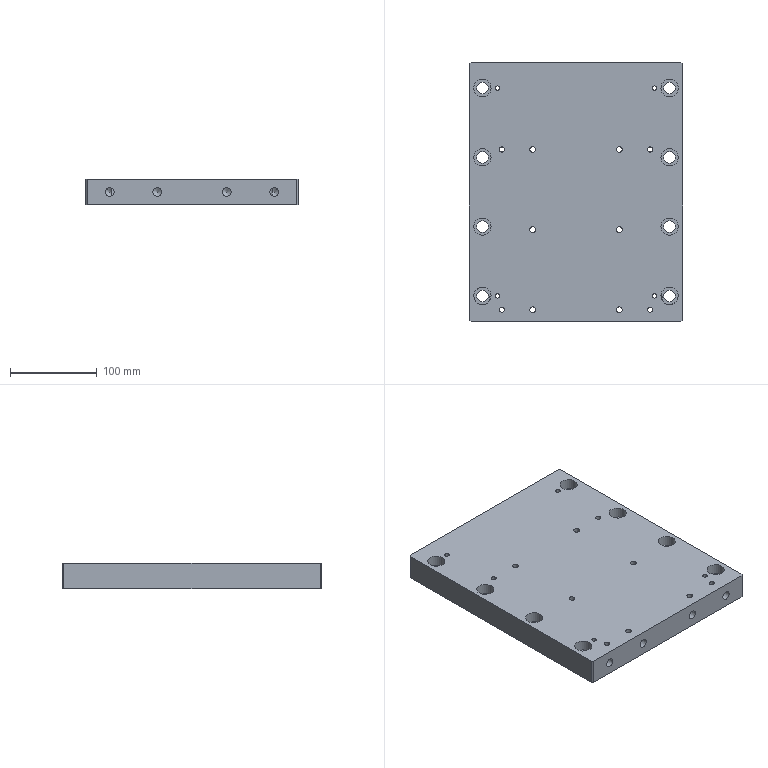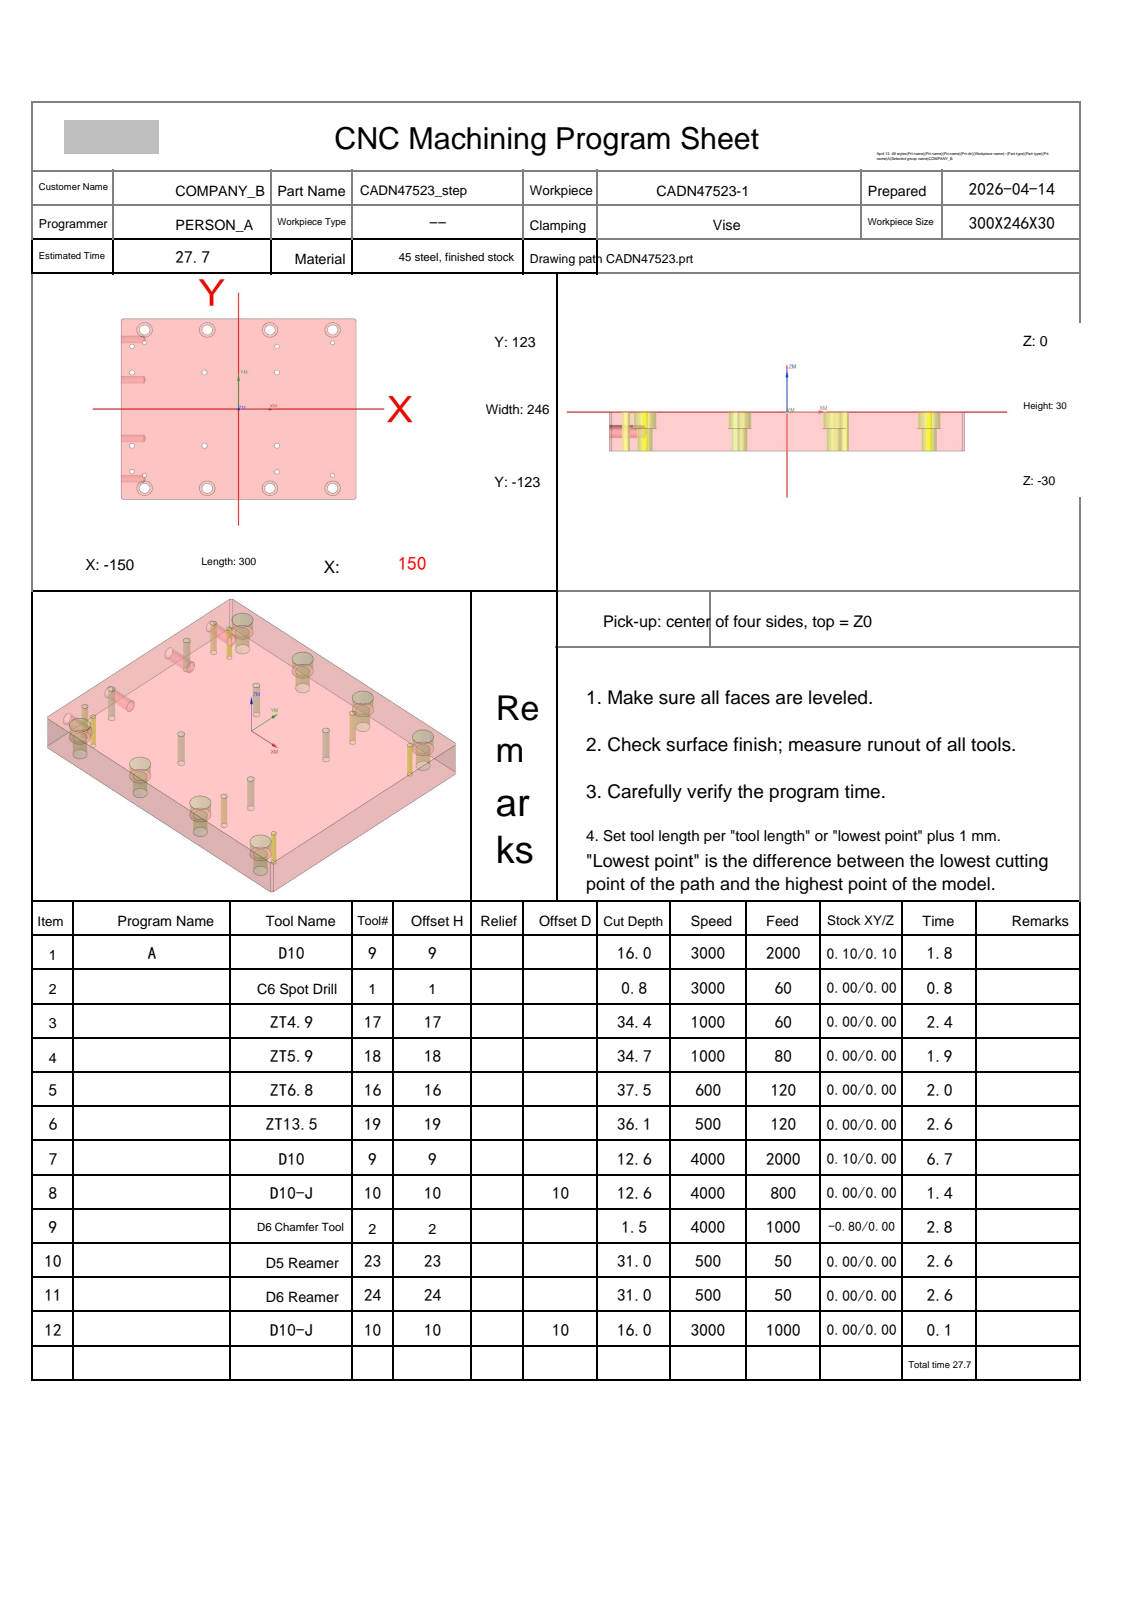NC program | NX | posted by the shop | part box 246 x 300 x 30 mm
Whole program, first 1647 of 1998 lines:
%
O0001
(Machine time: 29.90 MIN)
(===Total Tool:10===)
(T9=D10     D=10.  R=0.   D-  H09 Z=-16.  )
(T1=C6 Spot Drill   D=6.   R=0.   D-  H01 Z=-0.8  )
(T17=ZT4.9  D=4.9  DR_a=120 D-  H17 Z=-34.41)
(T18=ZT5.9  D=5.9  DR_a=120 D-  H18 Z=-34.7 )
(T16=ZT6.8  D=6.8  DR_a=118 D-  H16 Z=-37.54)
(T19=ZT13.5 D=13.5 DR_a=118 D-  H19 Z=-36.06)
(T10=D10-J  D=10.  R=0.   D10 H10 Z=-16.  )
(T2=D6 Chamfer Tool   D=6.   R=0.   D-  H02 Z=-1.5  )
(T23=D5 Reamer   D=5.   DR_a=180 D-  H23 Z=-31.  )
(T24=D6 Reamer   D=6.   DR_a=180 D-  H24 Z=-31.  )
G80 G90 G17 G49 G40
G91 G28 Z0
M01
N1 T09 M06
(D10  D=10. R=0. H=09 ce=0.10 di=0.10)
G00 G90 G54 X145.112 Y133.1 M03 S3000
G43 H09 Z20.
M08
Z-.4
G01 X151.606 Y126.606 F2000.
X153.606 Y124.606
X160.1 Y118.112
G00 Z-.8
G01 X153.606 Y124.606
X151.606 Y126.606
X145.112 Y133.1
G00 Z-1.2
G01 X151.606 Y126.606
X153.606 Y124.606
X160.1 Y118.112
G00 Z-1.6
G01 X153.606 Y124.606
X151.606 Y126.606
X145.112 Y133.1
G00 Z-2.
G01 X151.606 Y126.606
X153.606 Y124.606
X160.1 Y118.112
G00 Z-2.4
G01 X153.606 Y124.606
X151.606 Y126.606
X145.112 Y133.1
G00 Z-2.8
G01 X151.606 Y126.606
X153.606 Y124.606
X160.1 Y118.112
G00 Z-3.2
G01 X153.606 Y124.606
X151.606 Y126.606
X145.112 Y133.1
G00 Z-3.6
G01 X151.606 Y126.606
X153.606 Y124.606
X160.1 Y118.112
G00 Z-4.
G01 X153.606 Y124.606
X151.606 Y126.606
X145.112 Y133.1
G00 Z-4.4
G01 X151.606 Y126.606
X153.606 Y124.606
X160.1 Y118.112
G00 Z-4.8
G01 X153.606 Y124.606
X151.606 Y126.606
X145.112 Y133.1
G00 Z-5.2
G01 X151.606 Y126.606
X153.606 Y124.606
X160.1 Y118.112
G00 Z-5.6
G01 X153.606 Y124.606
X151.606 Y126.606
X145.112 Y133.1
G00 Z-6.
G01 X151.606 Y126.606
X153.606 Y124.606
X160.1 Y118.112
G00 Z-6.4
G01 X153.606 Y124.606
X151.606 Y126.606
X145.112 Y133.1
G00 Z-6.8
G01 X151.606 Y126.606
X153.606 Y124.606
X160.1 Y118.112
G00 Z-7.2
G01 X153.606 Y124.606
X151.606 Y126.606
X145.112 Y133.1
G00 Z-7.6
G01 X151.606 Y126.606
X153.606 Y124.606
X160.1 Y118.112
G00 Z-8.
G01 X153.606 Y124.606
X151.606 Y126.606
X145.112 Y133.1
G00 Z-8.4
G01 X151.606 Y126.606
X153.606 Y124.606
X160.1 Y118.112
G00 Z-8.8
G01 X153.606 Y124.606
X151.606 Y126.606
X145.112 Y133.1
G00 Z-9.2
G01 X151.606 Y126.606
X153.606 Y124.606
X160.1 Y118.112
G00 Z-9.6
G01 X153.606 Y124.606
X151.606 Y126.606
X145.112 Y133.1
G00 Z-10.
G01 X151.606 Y126.606
X153.606 Y124.606
X160.1 Y118.112
G00 Z-10.4
G01 X153.606 Y124.606
X151.606 Y126.606
X145.112 Y133.1
G00 Z-10.8
G01 X151.606 Y126.606
X153.606 Y124.606
X160.1 Y118.112
G00 Z-11.2
G01 X153.606 Y124.606
X151.606 Y126.606
X145.112 Y133.1
G00 Z-11.6
G01 X151.606 Y126.606
X153.606 Y124.606
X160.1 Y118.112
G00 Z-12.
G01 X153.606 Y124.606
X151.606 Y126.606
X145.112 Y133.1
G00 Z-12.4
G01 X151.606 Y126.606
X153.606 Y124.606
X160.1 Y118.112
G00 Z-12.8
G01 X153.606 Y124.606
X151.606 Y126.606
X145.112 Y133.1
G00 Z-13.2
G01 X151.606 Y126.606
X153.606 Y124.606
X160.1 Y118.112
G00 Z-13.6
G01 X153.606 Y124.606
X151.606 Y126.606
X145.112 Y133.1
G00 Z-14.
G01 X151.606 Y126.606
X153.606 Y124.606
X160.1 Y118.112
G00 Z-14.4
G01 X153.606 Y124.606
X151.606 Y126.606
X145.112 Y133.1
G00 Z-14.8
G01 X151.606 Y126.606
X153.606 Y124.606
X160.1 Y118.112
G00 Z-15.2
G01 X153.606 Y124.606
X151.606 Y126.606
X145.112 Y133.1
G00 Z-15.6
G01 X151.606 Y126.606
X153.606 Y124.606
X160.1 Y118.112
G00 Z-16.
G01 X153.606 Y124.606
X151.606 Y126.606
X145.112 Y133.1
G00 Z20.
X160.1 Y-118.112
Z-.4
G01 X153.606 Y-124.606
X151.606 Y-126.606
X145.112 Y-133.1
G00 Z-.8
G01 X151.606 Y-126.606
X153.606 Y-124.606
X160.1 Y-118.112
G00 Z-1.2
G01 X153.606 Y-124.606
X151.606 Y-126.606
X145.112 Y-133.1
G00 Z-1.6
G01 X151.606 Y-126.606
X153.606 Y-124.606
X160.1 Y-118.112
G00 Z-2.
G01 X153.606 Y-124.606
X151.606 Y-126.606
X145.112 Y-133.1
G00 Z-2.4
G01 X151.606 Y-126.606
X153.606 Y-124.606
X160.1 Y-118.112
G00 Z-2.8
G01 X153.606 Y-124.606
X151.606 Y-126.606
X145.112 Y-133.1
G00 Z-3.2
G01 X151.606 Y-126.606
X153.606 Y-124.606
X160.1 Y-118.112
G00 Z-3.6
G01 X153.606 Y-124.606
X151.606 Y-126.606
X145.112 Y-133.1
G00 Z-4.
G01 X151.606 Y-126.606
X153.606 Y-124.606
X160.1 Y-118.112
G00 Z-4.4
G01 X153.606 Y-124.606
X151.606 Y-126.606
X145.112 Y-133.1
G00 Z-4.8
G01 X151.606 Y-126.606
X153.606 Y-124.606
X160.1 Y-118.112
G00 Z-5.2
G01 X153.606 Y-124.606
X151.606 Y-126.606
X145.112 Y-133.1
G00 Z-5.6
G01 X151.606 Y-126.606
X153.606 Y-124.606
X160.1 Y-118.112
G00 Z-6.
G01 X153.606 Y-124.606
X151.606 Y-126.606
X145.112 Y-133.1
G00 Z-6.4
G01 X151.606 Y-126.606
X153.606 Y-124.606
X160.1 Y-118.112
G00 Z-6.8
G01 X153.606 Y-124.606
X151.606 Y-126.606
X145.112 Y-133.1
G00 Z-7.2
G01 X151.606 Y-126.606
X153.606 Y-124.606
X160.1 Y-118.112
G00 Z-7.6
G01 X153.606 Y-124.606
X151.606 Y-126.606
X145.112 Y-133.1
G00 Z-8.
G01 X151.606 Y-126.606
X153.606 Y-124.606
X160.1 Y-118.112
G00 Z-8.4
G01 X153.606 Y-124.606
X151.606 Y-126.606
X145.112 Y-133.1
G00 Z-8.8
G01 X151.606 Y-126.606
X153.606 Y-124.606
X160.1 Y-118.112
G00 Z-9.2
G01 X153.606 Y-124.606
X151.606 Y-126.606
X145.112 Y-133.1
G00 Z-9.6
G01 X151.606 Y-126.606
X153.606 Y-124.606
X160.1 Y-118.112
G00 Z-10.
G01 X153.606 Y-124.606
X151.606 Y-126.606
X145.112 Y-133.1
G00 Z-10.4
G01 X151.606 Y-126.606
X153.606 Y-124.606
X160.1 Y-118.112
G00 Z-10.8
G01 X153.606 Y-124.606
X151.606 Y-126.606
X145.112 Y-133.1
G00 Z-11.2
G01 X151.606 Y-126.606
X153.606 Y-124.606
X160.1 Y-118.112
G00 Z-11.6
G01 X153.606 Y-124.606
X151.606 Y-126.606
X145.112 Y-133.1
G00 Z-12.
G01 X151.606 Y-126.606
X153.606 Y-124.606
X160.1 Y-118.112
G00 Z-12.4
G01 X153.606 Y-124.606
X151.606 Y-126.606
X145.112 Y-133.1
G00 Z-12.8
G01 X151.606 Y-126.606
X153.606 Y-124.606
X160.1 Y-118.112
G00 Z-13.2
G01 X153.606 Y-124.606
X151.606 Y-126.606
X145.112 Y-133.1
G00 Z-13.6
G01 X151.606 Y-126.606
X153.606 Y-124.606
X160.1 Y-118.112
G00 Z-14.
G01 X153.606 Y-124.606
X151.606 Y-126.606
X145.112 Y-133.1
G00 Z-14.4
G01 X151.606 Y-126.606
X153.606 Y-124.606
X160.1 Y-118.112
G00 Z-14.8
G01 X153.606 Y-124.606
X151.606 Y-126.606
X145.112 Y-133.1
G00 Z-15.2
G01 X151.606 Y-126.606
X153.606 Y-124.606
X160.1 Y-118.112
G00 Z-15.6
G01 X153.606 Y-124.606
X151.606 Y-126.606
X145.112 Y-133.1
G00 Z-16.
G01 X151.606 Y-126.606
X153.606 Y-124.606
X160.1 Y-118.112
G00 Z20.
X-145.112 Y-133.1
Z-.4
G01 X-151.606 Y-126.606
X-153.606 Y-124.606
X-160.1 Y-118.112
G00 Z-.8
G01 X-153.606 Y-124.606
X-151.606 Y-126.606
X-145.112 Y-133.1
G00 Z-1.2
G01 X-151.606 Y-126.606
X-153.606 Y-124.606
X-160.1 Y-118.112
G00 Z-1.6
G01 X-153.606 Y-124.606
X-151.606 Y-126.606
X-145.112 Y-133.1
G00 Z-2.
G01 X-151.606 Y-126.606
X-153.606 Y-124.606
X-160.1 Y-118.112
G00 Z-2.4
G01 X-153.606 Y-124.606
X-151.606 Y-126.606
X-145.112 Y-133.1
G00 Z-2.8
G01 X-151.606 Y-126.606
X-153.606 Y-124.606
X-160.1 Y-118.112
G00 Z-3.2
G01 X-153.606 Y-124.606
X-151.606 Y-126.606
X-145.112 Y-133.1
G00 Z-3.6
G01 X-151.606 Y-126.606
X-153.606 Y-124.606
X-160.1 Y-118.112
G00 Z-4.
G01 X-153.606 Y-124.606
X-151.606 Y-126.606
X-145.112 Y-133.1
G00 Z-4.4
G01 X-151.606 Y-126.606
X-153.606 Y-124.606
X-160.1 Y-118.112
G00 Z-4.8
G01 X-153.606 Y-124.606
X-151.606 Y-126.606
X-145.112 Y-133.1
G00 Z-5.2
G01 X-151.606 Y-126.606
X-153.606 Y-124.606
X-160.1 Y-118.112
G00 Z-5.6
G01 X-153.606 Y-124.606
X-151.606 Y-126.606
X-145.112 Y-133.1
G00 Z-6.
G01 X-151.606 Y-126.606
X-153.606 Y-124.606
X-160.1 Y-118.112
G00 Z-6.4
G01 X-153.606 Y-124.606
X-151.606 Y-126.606
X-145.112 Y-133.1
G00 Z-6.8
G01 X-151.606 Y-126.606
X-153.606 Y-124.606
X-160.1 Y-118.112
G00 Z-7.2
G01 X-153.606 Y-124.606
X-151.606 Y-126.606
X-145.112 Y-133.1
G00 Z-7.6
G01 X-151.606 Y-126.606
X-153.606 Y-124.606
X-160.1 Y-118.112
G00 Z-8.
G01 X-153.606 Y-124.606
X-151.606 Y-126.606
X-145.112 Y-133.1
G00 Z-8.4
G01 X-151.606 Y-126.606
X-153.606 Y-124.606
X-160.1 Y-118.112
G00 Z-8.8
G01 X-153.606 Y-124.606
X-151.606 Y-126.606
X-145.112 Y-133.1
G00 Z-9.2
G01 X-151.606 Y-126.606
X-153.606 Y-124.606
X-160.1 Y-118.112
G00 Z-9.6
G01 X-153.606 Y-124.606
X-151.606 Y-126.606
X-145.112 Y-133.1
G00 Z-10.
G01 X-151.606 Y-126.606
X-153.606 Y-124.606
X-160.1 Y-118.112
G00 Z-10.4
G01 X-153.606 Y-124.606
X-151.606 Y-126.606
X-145.112 Y-133.1
G00 Z-10.8
G01 X-151.606 Y-126.606
X-153.606 Y-124.606
X-160.1 Y-118.112
G00 Z-11.2
G01 X-153.606 Y-124.606
X-151.606 Y-126.606
X-145.112 Y-133.1
G00 Z-11.6
G01 X-151.606 Y-126.606
X-153.606 Y-124.606
X-160.1 Y-118.112
G00 Z-12.
G01 X-153.606 Y-124.606
X-151.606 Y-126.606
X-145.112 Y-133.1
G00 Z-12.4
G01 X-151.606 Y-126.606
X-153.606 Y-124.606
X-160.1 Y-118.112
G00 Z-12.8
G01 X-153.606 Y-124.606
X-151.606 Y-126.606
X-145.112 Y-133.1
G00 Z-13.2
G01 X-151.606 Y-126.606
X-153.606 Y-124.606
X-160.1 Y-118.112
G00 Z-13.6
G01 X-153.606 Y-124.606
X-151.606 Y-126.606
X-145.112 Y-133.1
G00 Z-14.
G01 X-151.606 Y-126.606
X-153.606 Y-124.606
X-160.1 Y-118.112
G00 Z-14.4
G01 X-153.606 Y-124.606
X-151.606 Y-126.606
X-145.112 Y-133.1
G00 Z-14.8
G01 X-151.606 Y-126.606
X-153.606 Y-124.606
X-160.1 Y-118.112
G00 Z-15.2
G01 X-153.606 Y-124.606
X-151.606 Y-126.606
X-145.112 Y-133.1
G00 Z-15.6
G01 X-151.606 Y-126.606
X-153.606 Y-124.606
X-160.1 Y-118.112
G00 Z-16.
G01 X-153.606 Y-124.606
X-151.606 Y-126.606
X-145.112 Y-133.1
G00 Z20.
X-160.1 Y118.112
Z-.4
G01 X-153.606 Y124.606
X-151.606 Y126.606
X-145.112 Y133.1
G00 Z-.8
G01 X-151.606 Y126.606
X-153.606 Y124.606
X-160.1 Y118.112
G00 Z-1.2
G01 X-153.606 Y124.606
X-151.606 Y126.606
X-145.112 Y133.1
G00 Z-1.6
G01 X-151.606 Y126.606
X-153.606 Y124.606
X-160.1 Y118.112
G00 Z-2.
G01 X-153.606 Y124.606
X-151.606 Y126.606
X-145.112 Y133.1
G00 Z-2.4
G01 X-151.606 Y126.606
X-153.606 Y124.606
X-160.1 Y118.112
G00 Z-2.8
G01 X-153.606 Y124.606
X-151.606 Y126.606
X-145.112 Y133.1
G00 Z-3.2
G01 X-151.606 Y126.606
X-153.606 Y124.606
X-160.1 Y118.112
G00 Z-3.6
G01 X-153.606 Y124.606
X-151.606 Y126.606
X-145.112 Y133.1
G00 Z-4.
G01 X-151.606 Y126.606
X-153.606 Y124.606
X-160.1 Y118.112
G00 Z-4.4
G01 X-153.606 Y124.606
X-151.606 Y126.606
X-145.112 Y133.1
G00 Z-4.8
G01 X-151.606 Y126.606
X-153.606 Y124.606
X-160.1 Y118.112
G00 Z-5.2
G01 X-153.606 Y124.606
X-151.606 Y126.606
X-145.112 Y133.1
G00 Z-5.6
G01 X-151.606 Y126.606
X-153.606 Y124.606
X-160.1 Y118.112
G00 Z-6.
G01 X-153.606 Y124.606
X-151.606 Y126.606
X-145.112 Y133.1
G00 Z-6.4
G01 X-151.606 Y126.606
X-153.606 Y124.606
X-160.1 Y118.112
G00 Z-6.8
G01 X-153.606 Y124.606
X-151.606 Y126.606
X-145.112 Y133.1
G00 Z-7.2
G01 X-151.606 Y126.606
X-153.606 Y124.606
X-160.1 Y118.112
G00 Z-7.6
G01 X-153.606 Y124.606
X-151.606 Y126.606
X-145.112 Y133.1
G00 Z-8.
G01 X-151.606 Y126.606
X-153.606 Y124.606
X-160.1 Y118.112
G00 Z-8.4
G01 X-153.606 Y124.606
X-151.606 Y126.606
X-145.112 Y133.1
G00 Z-8.8
G01 X-151.606 Y126.606
X-153.606 Y124.606
X-160.1 Y118.112
G00 Z-9.2
G01 X-153.606 Y124.606
X-151.606 Y126.606
X-145.112 Y133.1
G00 Z-9.6
G01 X-151.606 Y126.606
X-153.606 Y124.606
X-160.1 Y118.112
G00 Z-10.
G01 X-153.606 Y124.606
X-151.606 Y126.606
X-145.112 Y133.1
G00 Z-10.4
G01 X-151.606 Y126.606
X-153.606 Y124.606
X-160.1 Y118.112
G00 Z-10.8
G01 X-153.606 Y124.606
X-151.606 Y126.606
X-145.112 Y133.1
G00 Z-11.2
G01 X-151.606 Y126.606
X-153.606 Y124.606
X-160.1 Y118.112
G00 Z-11.6
G01 X-153.606 Y124.606
X-151.606 Y126.606
X-145.112 Y133.1
G00 Z-12.
G01 X-151.606 Y126.606
X-153.606 Y124.606
X-160.1 Y118.112
G00 Z-12.4
G01 X-153.606 Y124.606
X-151.606 Y126.606
X-145.112 Y133.1
G00 Z-12.8
G01 X-151.606 Y126.606
X-153.606 Y124.606
X-160.1 Y118.112
G00 Z-13.2
G01 X-153.606 Y124.606
X-151.606 Y126.606
X-145.112 Y133.1
G00 Z-13.6
G01 X-151.606 Y126.606
X-153.606 Y124.606
X-160.1 Y118.112
G00 Z-14.
G01 X-153.606 Y124.606
X-151.606 Y126.606
X-145.112 Y133.1
G00 Z-14.4
G01 X-151.606 Y126.606
X-153.606 Y124.606
X-160.1 Y118.112
G00 Z-14.8
G01 X-153.606 Y124.606
X-151.606 Y126.606
X-145.112 Y133.1
G00 Z-15.2
G01 X-151.606 Y126.606
X-153.606 Y124.606
X-160.1 Y118.112
G00 Z-15.6
G01 X-153.606 Y124.606
X-151.606 Y126.606
X-145.112 Y133.1
G00 Z-16.
G01 X-151.606 Y126.606
X-153.606 Y124.606
X-160.1 Y118.112
G00 Z20.
G91 G28 Z0.0
M05
M09
G91 G28 Z0.0
M01
N2 T01 M06
(C6 Spot Drill  D=6. R=0. H=01 ce=0.00 di=0.10)
G00 G90 G54 X120. Y-90.5 M03 S3000
G43 H01 Z20.
M08
G98 G81 X120. Y-90.5 Z-.8 R1. F60.
Y-108.
X40.
X49. Y-85.5
Y-50.
X-43.5
X-40. Y-108.
X-120.
Y-90.5
X-136. Y-85.5
Y-50.
Y50.
Y85.5
X-120. Y90.5
Y108.
X-40.
X-43.5 Y50.
X49.
Y85.5
X40. Y108.
X120.
Y90.5
G80
G00 Z20.
G91 G28 Z0.0
M05
M09
G91 G28 Z0.0
M01
N3 T17 M06
(ZT4.9 D=4.9 DR_a=120 H=17)
G00 G90 G54 X-120. Y90.5 M03 S1000
G43 H17 Z20.
M08
G98 G83 X-120. Y90.5 Z-34.415 R1. F60. Q1.
Y-90.5
X120.
Y90.5
G80
G00 Z20.
G91 G28 Z0.0
M05
M09
G91 G28 Z0.0
M01
N4 T18 M06
(ZT5.9 D=5.9 DR_a=120 H=18)
G00 G90 G54 X-136. Y85.5 M03 S1000
G43 H18 Z20.
M08
G98 G83 X-136. Y85.5 Z-34.703 R1. F80. Q1.
Y-85.5
X49.
Y85.5
G80
G00 Z20.
G91 G28 Z0.0
M05
M09
G91 G28 Z0.0
M01
N5 T16 M06
(ZT6.8 D=6.8 DR_a=118 H=16)
G00 G90 G54 X49. Y-50. M03 S600
G43 H16 Z20.
M08
G98 G83 X49. Y-50. Z-37.543 R1. F120. Q2.
X-43.5
X-136.
Y50.
X-43.5
X49.
G80
G00 Z20.
G91 G28 Z0.0
M05
M09
G91 G28 Z0.0
M01
N6 T19 M06
(ZT13.5 D=13.5 DR_a=118 H=19)
G00 G90 G54 X120. Y108. M03 S500
G43 H19 Z20.
M08
G98 G83 X120. Y108. Z-36.056 R1. F120. Q2.
X40.
X-40.
X-120.
Y-108.
X-40.
X40.
X120.
G80
G00 Z20.
G91 G28 Z0.0
M05
M09
G91 G28 Z0.0
M01
N7 T09 M06
(D10  D=10. R=0. H=09 ce=0.10 di=0.00)
G00 G90 G54 X120. Y-108. M03 S4000
G43 H09 Z20.
M08
Z.5
G03 X117.55 Y-110.45 I0.0 J-2.45 F2000.
X120. Y-112.9 I2.45 J0.0
X120. Y-112.9 Z.25 I0.0 J4.9
X120. Y-112.9 Z0.0 I0.0 J4.9
X120. Y-112.9 Z-.25 I0.0 J4.9
X120. Y-112.9 Z-.5 I0.0 J4.9
X120. Y-112.9 Z-.75 I0.0 J4.9
X120. Y-112.9 Z-1. I0.0 J4.9
X120. Y-112.9 Z-1.25 I0.0 J4.9
X120. Y-112.9 Z-1.5 I0.0 J4.9
X120. Y-112.9 Z-1.75 I0.0 J4.9
X120. Y-112.9 Z-2. I0.0 J4.9
X120. Y-112.9 Z-2.25 I0.0 J4.9
X120. Y-112.9 Z-2.5 I0.0 J4.9
X120. Y-112.9 Z-2.75 I0.0 J4.9
X120. Y-112.9 Z-3. I0.0 J4.9
X120. Y-112.9 Z-3.25 I0.0 J4.9
X120. Y-112.9 Z-3.5 I0.0 J4.9
X120. Y-112.9 Z-3.75 I0.0 J4.9
X120. Y-112.9 Z-4. I0.0 J4.9
X120. Y-112.9 Z-4.25 I0.0 J4.9
X120. Y-112.9 Z-4.5 I0.0 J4.9
X120. Y-112.9 Z-4.75 I0.0 J4.9
X120. Y-112.9 Z-5. I0.0 J4.9
X120. Y-112.9 Z-5.25 I0.0 J4.9
X120. Y-112.9 Z-5.5 I0.0 J4.9
X120. Y-112.9 Z-5.75 I0.0 J4.9
X120. Y-112.9 Z-6. I0.0 J4.9
X120. Y-112.9 Z-6.25 I0.0 J4.9
X120. Y-112.9 Z-6.5 I0.0 J4.9
X120. Y-112.9 Z-6.75 I0.0 J4.9
X120. Y-112.9 Z-7. I0.0 J4.9
X120. Y-112.9 Z-7.25 I0.0 J4.9
X120. Y-112.9 Z-7.5 I0.0 J4.9
X120. Y-112.9 Z-7.75 I0.0 J4.9
X120. Y-112.9 Z-8. I0.0 J4.9
X120. Y-112.9 Z-8.25 I0.0 J4.9
X120. Y-112.9 Z-8.5 I0.0 J4.9
X120. Y-112.9 Z-8.75 I0.0 J4.9
X120. Y-112.9 Z-9. I0.0 J4.9
X120. Y-112.9 Z-9.25 I0.0 J4.9
X120. Y-112.9 Z-9.5 I0.0 J4.9
X120. Y-112.9 Z-9.75 I0.0 J4.9
X120. Y-112.9 Z-10. I0.0 J4.9
X120. Y-112.9 Z-10.25 I0.0 J4.9
X120. Y-112.9 Z-10.5 I0.0 J4.9
X120. Y-112.9 Z-10.75 I0.0 J4.9
X120. Y-112.9 Z-11. I0.0 J4.9
X120. Y-112.9 Z-11.25 I0.0 J4.9
X120. Y-112.9 Z-11.5 I0.0 J4.9
X120. Y-112.9 Z-11.75 I0.0 J4.9
X120. Y-112.9 Z-12. I0.0 J4.9
X120. Y-112.9 Z-12.25 I0.0 J4.9
X120. Y-112.9 Z-12.5 I0.0 J4.9
X122.88 Y-104.036 Z-12.6 I0.0 J4.9
X120. Y-103.1 I-2.88 J-3.964
X115.1 Y-108. I0.0 J-4.9
X120. Y-112.9 I4.9 J0.0
X124.9 Y-108. I0.0 J4.9
X122.88 Y-104.036 I-4.9 J0.0
X121.44 Y-103.568 I-1.44 J-1.982
X118.99 Y-106.018 I0.0 J-2.45
X120. Y-108. I2.45 J0.0
G00 Z20.
X40.
Z.5
G03 X37.55 Y-110.45 I0.0 J-2.45
X40. Y-112.9 I2.45 J0.0
X40. Y-112.9 Z.25 I0.0 J4.9
X40. Y-112.9 Z0.0 I0.0 J4.9
X40. Y-112.9 Z-.25 I0.0 J4.9
X40. Y-112.9 Z-.5 I0.0 J4.9
X40. Y-112.9 Z-.75 I0.0 J4.9
X40. Y-112.9 Z-1. I0.0 J4.9
X40. Y-112.9 Z-1.25 I0.0 J4.9
X40. Y-112.9 Z-1.5 I0.0 J4.9
X40. Y-112.9 Z-1.75 I0.0 J4.9
X40. Y-112.9 Z-2. I0.0 J4.9
X40. Y-112.9 Z-2.25 I0.0 J4.9
X40. Y-112.9 Z-2.5 I0.0 J4.9
X40. Y-112.9 Z-2.75 I0.0 J4.9
X40. Y-112.9 Z-3. I0.0 J4.9
X40. Y-112.9 Z-3.25 I0.0 J4.9
X40. Y-112.9 Z-3.5 I0.0 J4.9
X40. Y-112.9 Z-3.75 I0.0 J4.9
X40. Y-112.9 Z-4. I0.0 J4.9
X40. Y-112.9 Z-4.25 I0.0 J4.9
X40. Y-112.9 Z-4.5 I0.0 J4.9
X40. Y-112.9 Z-4.75 I0.0 J4.9
X40. Y-112.9 Z-5. I0.0 J4.9
X40. Y-112.9 Z-5.25 I0.0 J4.9
X40. Y-112.9 Z-5.5 I0.0 J4.9
X40. Y-112.9 Z-5.75 I0.0 J4.9
X40. Y-112.9 Z-6. I0.0 J4.9
X40. Y-112.9 Z-6.25 I0.0 J4.9
X40. Y-112.9 Z-6.5 I0.0 J4.9
X40. Y-112.9 Z-6.75 I0.0 J4.9
X40. Y-112.9 Z-7. I0.0 J4.9
X40. Y-112.9 Z-7.25 I0.0 J4.9
X40. Y-112.9 Z-7.5 I0.0 J4.9
X40. Y-112.9 Z-7.75 I0.0 J4.9
X40. Y-112.9 Z-8. I0.0 J4.9
X40. Y-112.9 Z-8.25 I0.0 J4.9
X40. Y-112.9 Z-8.5 I0.0 J4.9
X40. Y-112.9 Z-8.75 I0.0 J4.9
X40. Y-112.9 Z-9. I0.0 J4.9
X40. Y-112.9 Z-9.25 I0.0 J4.9
X40. Y-112.9 Z-9.5 I0.0 J4.9
X40. Y-112.9 Z-9.75 I0.0 J4.9
X40. Y-112.9 Z-10. I0.0 J4.9
X40. Y-112.9 Z-10.25 I0.0 J4.9
X40. Y-112.9 Z-10.5 I0.0 J4.9
X40. Y-112.9 Z-10.75 I0.0 J4.9
X40. Y-112.9 Z-11. I0.0 J4.9
X40. Y-112.9 Z-11.25 I0.0 J4.9
X40. Y-112.9 Z-11.5 I0.0 J4.9
X40. Y-112.9 Z-11.75 I0.0 J4.9
X40. Y-112.9 Z-12. I0.0 J4.9
X40. Y-112.9 Z-12.25 I0.0 J4.9
X40. Y-112.9 Z-12.5 I0.0 J4.9
X42.88 Y-104.036 Z-12.6 I0.0 J4.9
X40. Y-103.1 I-2.88 J-3.964
X35.1 Y-108. I0.0 J-4.9
X40. Y-112.9 I4.9 J0.0
X44.9 Y-108. I0.0 J4.9
X42.88 Y-104.036 I-4.9 J0.0
X41.44 Y-103.568 I-1.44 J-1.982
X38.99 Y-106.018 I0.0 J-2.45
X40. Y-108. I2.45 J0.0
G00 Z20.
X-40.
Z.5
G03 X-42.45 Y-110.45 I0.0 J-2.45
X-40. Y-112.9 I2.45 J0.0
X-40. Y-112.9 Z.25 I0.0 J4.9
X-40. Y-112.9 Z0.0 I0.0 J4.9
X-40. Y-112.9 Z-.25 I0.0 J4.9
X-40. Y-112.9 Z-.5 I0.0 J4.9
X-40. Y-112.9 Z-.75 I0.0 J4.9
X-40. Y-112.9 Z-1. I0.0 J4.9
X-40. Y-112.9 Z-1.25 I0.0 J4.9
X-40. Y-112.9 Z-1.5 I0.0 J4.9
X-40. Y-112.9 Z-1.75 I0.0 J4.9
X-40. Y-112.9 Z-2. I0.0 J4.9
X-40. Y-112.9 Z-2.25 I0.0 J4.9
X-40. Y-112.9 Z-2.5 I0.0 J4.9
X-40. Y-112.9 Z-2.75 I0.0 J4.9
X-40. Y-112.9 Z-3. I0.0 J4.9
X-40. Y-112.9 Z-3.25 I0.0 J4.9
X-40. Y-112.9 Z-3.5 I0.0 J4.9
X-40. Y-112.9 Z-3.75 I0.0 J4.9
X-40. Y-112.9 Z-4. I0.0 J4.9
X-40. Y-112.9 Z-4.25 I0.0 J4.9
X-40. Y-112.9 Z-4.5 I0.0 J4.9
X-40. Y-112.9 Z-4.75 I0.0 J4.9
X-40. Y-112.9 Z-5. I0.0 J4.9
X-40. Y-112.9 Z-5.25 I0.0 J4.9
X-40. Y-112.9 Z-5.5 I0.0 J4.9
X-40. Y-112.9 Z-5.75 I0.0 J4.9
X-40. Y-112.9 Z-6. I0.0 J4.9
X-40. Y-112.9 Z-6.25 I0.0 J4.9
X-40. Y-112.9 Z-6.5 I0.0 J4.9
X-40. Y-112.9 Z-6.75 I0.0 J4.9
X-40. Y-112.9 Z-7. I0.0 J4.9
X-40. Y-112.9 Z-7.25 I0.0 J4.9
X-40. Y-112.9 Z-7.5 I0.0 J4.9
X-40. Y-112.9 Z-7.75 I0.0 J4.9
X-40. Y-112.9 Z-8. I0.0 J4.9
X-40. Y-112.9 Z-8.25 I0.0 J4.9
X-40. Y-112.9 Z-8.5 I0.0 J4.9
X-40. Y-112.9 Z-8.75 I0.0 J4.9
X-40. Y-112.9 Z-9. I0.0 J4.9
X-40. Y-112.9 Z-9.25 I0.0 J4.9
X-40. Y-112.9 Z-9.5 I0.0 J4.9
X-40. Y-112.9 Z-9.75 I0.0 J4.9
X-40. Y-112.9 Z-10. I0.0 J4.9
X-40. Y-112.9 Z-10.25 I0.0 J4.9
X-40. Y-112.9 Z-10.5 I0.0 J4.9
X-40. Y-112.9 Z-10.75 I0.0 J4.9
X-40. Y-112.9 Z-11. I0.0 J4.9
X-40. Y-112.9 Z-11.25 I0.0 J4.9
X-40. Y-112.9 Z-11.5 I0.0 J4.9
X-40. Y-112.9 Z-11.75 I0.0 J4.9
X-40. Y-112.9 Z-12. I0.0 J4.9
X-40. Y-112.9 Z-12.25 I0.0 J4.9
X-40. Y-112.9 Z-12.5 I0.0 J4.9
X-37.12 Y-104.036 Z-12.6 I0.0 J4.9
X-40. Y-103.1 I-2.88 J-3.964
X-44.9 Y-108. I0.0 J-4.9
X-40. Y-112.9 I4.9 J0.0
X-35.1 Y-108. I0.0 J4.9
X-37.12 Y-104.036 I-4.9 J0.0
X-38.56 Y-103.568 I-1.44 J-1.982
X-41.01 Y-106.018 I0.0 J-2.45
X-40. Y-108. I2.45 J0.0
G00 Z20.
X-120.
Z.5
G03 X-122.45 Y-110.45 I0.0 J-2.45
X-120. Y-112.9 I2.45 J0.0
X-120. Y-112.9 Z.25 I0.0 J4.9
X-120. Y-112.9 Z0.0 I0.0 J4.9
X-120. Y-112.9 Z-.25 I0.0 J4.9
X-120. Y-112.9 Z-.5 I0.0 J4.9
X-120. Y-112.9 Z-.75 I0.0 J4.9
X-120. Y-112.9 Z-1. I0.0 J4.9
X-120. Y-112.9 Z-1.25 I0.0 J4.9
X-120. Y-112.9 Z-1.5 I0.0 J4.9
X-120. Y-112.9 Z-1.75 I0.0 J4.9
X-120. Y-112.9 Z-2. I0.0 J4.9
X-120. Y-112.9 Z-2.25 I0.0 J4.9
X-120. Y-112.9 Z-2.5 I0.0 J4.9
X-120. Y-112.9 Z-2.75 I0.0 J4.9
X-120. Y-112.9 Z-3. I0.0 J4.9
X-120. Y-112.9 Z-3.25 I0.0 J4.9
X-120. Y-112.9 Z-3.5 I0.0 J4.9
X-120. Y-112.9 Z-3.75 I0.0 J4.9
X-120. Y-112.9 Z-4. I0.0 J4.9
X-120. Y-112.9 Z-4.25 I0.0 J4.9
X-120. Y-112.9 Z-4.5 I0.0 J4.9
X-120. Y-112.9 Z-4.75 I0.0 J4.9
X-120. Y-112.9 Z-5. I0.0 J4.9
X-120. Y-112.9 Z-5.25 I0.0 J4.9
X-120. Y-112.9 Z-5.5 I0.0 J4.9
X-120. Y-112.9 Z-5.75 I0.0 J4.9
X-120. Y-112.9 Z-6. I0.0 J4.9
X-120. Y-112.9 Z-6.25 I0.0 J4.9
X-120. Y-112.9 Z-6.5 I0.0 J4.9
X-120. Y-112.9 Z-6.75 I0.0 J4.9
X-120. Y-112.9 Z-7. I0.0 J4.9
X-120. Y-112.9 Z-7.25 I0.0 J4.9
X-120. Y-112.9 Z-7.5 I0.0 J4.9
X-120. Y-112.9 Z-7.75 I0.0 J4.9
X-120. Y-112.9 Z-8. I0.0 J4.9
X-120. Y-112.9 Z-8.25 I0.0 J4.9
X-120. Y-112.9 Z-8.5 I0.0 J4.9
X-120. Y-112.9 Z-8.75 I0.0 J4.9
X-120. Y-112.9 Z-9. I0.0 J4.9
X-120. Y-112.9 Z-9.25 I0.0 J4.9
X-120. Y-112.9 Z-9.5 I0.0 J4.9
X-120. Y-112.9 Z-9.75 I0.0 J4.9
X-120. Y-112.9 Z-10. I0.0 J4.9
X-120. Y-112.9 Z-10.25 I0.0 J4.9
X-120. Y-112.9 Z-10.5 I0.0 J4.9
X-120. Y-112.9 Z-10.75 I0.0 J4.9
X-120. Y-112.9 Z-11. I0.0 J4.9
X-120. Y-112.9 Z-11.25 I0.0 J4.9
X-120. Y-112.9 Z-11.5 I0.0 J4.9
X-120. Y-112.9 Z-11.75 I0.0 J4.9
X-120. Y-112.9 Z-12. I0.0 J4.9
X-120. Y-112.9 Z-12.25 I0.0 J4.9
X-120. Y-112.9 Z-12.5 I0.0 J4.9
X-117.12 Y-104.036 Z-12.6 I0.0 J4.9
X-120. Y-103.1 I-2.88 J-3.964
X-124.9 Y-108. I0.0 J-4.9
X-120. Y-112.9 I4.9 J0.0
X-115.1 Y-108. I0.0 J4.9
X-117.12 Y-104.036 I-4.9 J0.0
X-118.56 Y-103.568 I-1.44 J-1.982
X-121.01 Y-106.018 I0.0 J-2.45
X-120. Y-108. I2.45 J0.0
G00 Z20.
Y108.
Z.5
G03 X-122.45 Y105.55 I0.0 J-2.45
X-120. Y103.1 I2.45 J0.0
X-120. Y103.1 Z.25 I0.0 J4.9
X-120. Y103.1 Z0.0 I0.0 J4.9
X-120. Y103.1 Z-.25 I0.0 J4.9
X-120. Y103.1 Z-.5 I0.0 J4.9
X-120. Y103.1 Z-.75 I0.0 J4.9
X-120. Y103.1 Z-1. I0.0 J4.9
X-120. Y103.1 Z-1.25 I0.0 J4.9
X-120. Y103.1 Z-1.5 I0.0 J4.9
X-120. Y103.1 Z-1.75 I0.0 J4.9
X-120. Y103.1 Z-2. I0.0 J4.9
X-120. Y103.1 Z-2.25 I0.0 J4.9
X-120. Y103.1 Z-2.5 I0.0 J4.9
X-120. Y103.1 Z-2.75 I0.0 J4.9
X-120. Y103.1 Z-3. I0.0 J4.9
X-120. Y103.1 Z-3.25 I0.0 J4.9
X-120. Y103.1 Z-3.5 I0.0 J4.9
X-120. Y103.1 Z-3.75 I0.0 J4.9
X-120. Y103.1 Z-4. I0.0 J4.9
X-120. Y103.1 Z-4.25 I0.0 J4.9
X-120. Y103.1 Z-4.5 I0.0 J4.9
X-120. Y103.1 Z-4.75 I0.0 J4.9
X-120. Y103.1 Z-5. I0.0 J4.9
X-120. Y103.1 Z-5.25 I0.0 J4.9
X-120. Y103.1 Z-5.5 I0.0 J4.9
X-120. Y103.1 Z-5.75 I0.0 J4.9
X-120. Y103.1 Z-6. I0.0 J4.9
X-120. Y103.1 Z-6.25 I0.0 J4.9
X-120. Y103.1 Z-6.5 I0.0 J4.9
X-120. Y103.1 Z-6.75 I0.0 J4.9
X-120. Y103.1 Z-7. I0.0 J4.9
X-120. Y103.1 Z-7.25 I0.0 J4.9
X-120. Y103.1 Z-7.5 I0.0 J4.9
X-120. Y103.1 Z-7.75 I0.0 J4.9
X-120. Y103.1 Z-8. I0.0 J4.9
X-120. Y103.1 Z-8.25 I0.0 J4.9
X-120. Y103.1 Z-8.5 I0.0 J4.9
X-120. Y103.1 Z-8.75 I0.0 J4.9
X-120. Y103.1 Z-9. I0.0 J4.9
X-120. Y103.1 Z-9.25 I0.0 J4.9
X-120. Y103.1 Z-9.5 I0.0 J4.9
X-120. Y103.1 Z-9.75 I0.0 J4.9
X-120. Y103.1 Z-10. I0.0 J4.9
X-120. Y103.1 Z-10.25 I0.0 J4.9
X-120. Y103.1 Z-10.5 I0.0 J4.9
X-120. Y103.1 Z-10.75 I0.0 J4.9
X-120. Y103.1 Z-11. I0.0 J4.9
X-120. Y103.1 Z-11.25 I0.0 J4.9
X-120. Y103.1 Z-11.5 I0.0 J4.9
X-120. Y103.1 Z-11.75 I0.0 J4.9
X-120. Y103.1 Z-12. I0.0 J4.9
X-120. Y103.1 Z-12.25 I0.0 J4.9
X-120. Y103.1 Z-12.5 I0.0 J4.9
X-117.12 Y111.964 Z-12.6 I0.0 J4.9
X-120. Y112.9 I-2.88 J-3.964
X-124.9 Y108. I0.0 J-4.9
X-120. Y103.1 I4.9 J0.0
X-115.1 Y108. I0.0 J4.9
X-117.12 Y111.964 I-4.9 J0.0
X-118.56 Y112.432 I-1.44 J-1.982
X-121.01 Y109.982 I0.0 J-2.45
X-120. Y108. I2.45 J0.0
G00 Z20.
X-40.
Z.5
G03 X-42.45 Y105.55 I0.0 J-2.45
X-40. Y103.1 I2.45 J0.0
X-40. Y103.1 Z.25 I0.0 J4.9
X-40. Y103.1 Z0.0 I0.0 J4.9
X-40. Y103.1 Z-.25 I0.0 J4.9
X-40. Y103.1 Z-.5 I0.0 J4.9
X-40. Y103.1 Z-.75 I0.0 J4.9
X-40. Y103.1 Z-1. I0.0 J4.9
X-40. Y103.1 Z-1.25 I0.0 J4.9
X-40. Y103.1 Z-1.5 I0.0 J4.9
X-40. Y103.1 Z-1.75 I0.0 J4.9
X-40. Y103.1 Z-2. I0.0 J4.9
X-40. Y103.1 Z-2.25 I0.0 J4.9
X-40. Y103.1 Z-2.5 I0.0 J4.9
X-40. Y103.1 Z-2.75 I0.0 J4.9
X-40. Y103.1 Z-3. I0.0 J4.9
X-40. Y103.1 Z-3.25 I0.0 J4.9
X-40. Y103.1 Z-3.5 I0.0 J4.9
X-40. Y103.1 Z-3.75 I0.0 J4.9
X-40. Y103.1 Z-4. I0.0 J4.9
X-40. Y103.1 Z-4.25 I0.0 J4.9
X-40. Y103.1 Z-4.5 I0.0 J4.9
X-40. Y103.1 Z-4.75 I0.0 J4.9
X-40. Y103.1 Z-5. I0.0 J4.9
X-40. Y103.1 Z-5.25 I0.0 J4.9
X-40. Y103.1 Z-5.5 I0.0 J4.9
X-40. Y103.1 Z-5.75 I0.0 J4.9
X-40. Y103.1 Z-6. I0.0 J4.9
X-40. Y103.1 Z-6.25 I0.0 J4.9
X-40. Y103.1 Z-6.5 I0.0 J4.9
X-40. Y103.1 Z-6.75 I0.0 J4.9
X-40. Y103.1 Z-7. I0.0 J4.9
X-40. Y103.1 Z-7.25 I0.0 J4.9
X-40. Y103.1 Z-7.5 I0.0 J4.9
X-40. Y103.1 Z-7.75 I0.0 J4.9
X-40. Y103.1 Z-8. I0.0 J4.9
X-40. Y103.1 Z-8.25 I0.0 J4.9
X-40. Y103.1 Z-8.5 I0.0 J4.9
X-40. Y103.1 Z-8.75 I0.0 J4.9
X-40. Y103.1 Z-9. I0.0 J4.9
X-40. Y103.1 Z-9.25 I0.0 J4.9
X-40. Y103.1 Z-9.5 I0.0 J4.9
X-40. Y103.1 Z-9.75 I0.0 J4.9
X-40. Y103.1 Z-10. I0.0 J4.9
X-40. Y103.1 Z-10.25 I0.0 J4.9
X-40. Y103.1 Z-10.5 I0.0 J4.9
X-40. Y103.1 Z-10.75 I0.0 J4.9
X-40. Y103.1 Z-11. I0.0 J4.9
X-40. Y103.1 Z-11.25 I0.0 J4.9
X-40. Y103.1 Z-11.5 I0.0 J4.9
X-40. Y103.1 Z-11.75 I0.0 J4.9
X-40. Y103.1 Z-12. I0.0 J4.9
X-40. Y103.1 Z-12.25 I0.0 J4.9
X-40. Y103.1 Z-12.5 I0.0 J4.9
X-37.12 Y111.964 Z-12.6 I0.0 J4.9
X-40. Y112.9 I-2.88 J-3.964
X-44.9 Y108. I0.0 J-4.9
X-40. Y103.1 I4.9 J0.0
X-35.1 Y108. I0.0 J4.9
X-37.12 Y111.964 I-4.9 J0.0
X-38.56 Y112.432 I-1.44 J-1.982
X-41.01 Y109.982 I0.0 J-2.45
X-40. Y108. I2.45 J0.0
G00 Z20.
X40.
Z.5
G03 X37.55 Y105.55 I0.0 J-2.45
X40. Y103.1 I2.45 J0.0
X40. Y103.1 Z.25 I0.0 J4.9
X40. Y103.1 Z0.0 I0.0 J4.9
X40. Y103.1 Z-.25 I0.0 J4.9
X40. Y103.1 Z-.5 I0.0 J4.9
X40. Y103.1 Z-.75 I0.0 J4.9
X40. Y103.1 Z-1. I0.0 J4.9
X40. Y103.1 Z-1.25 I0.0 J4.9
X40. Y103.1 Z-1.5 I0.0 J4.9
X40. Y103.1 Z-1.75 I0.0 J4.9
X40. Y103.1 Z-2. I0.0 J4.9
X40. Y103.1 Z-2.25 I0.0 J4.9
X40. Y103.1 Z-2.5 I0.0 J4.9
X40. Y103.1 Z-2.75 I0.0 J4.9
X40. Y103.1 Z-3. I0.0 J4.9
X40. Y103.1 Z-3.25 I0.0 J4.9
X40. Y103.1 Z-3.5 I0.0 J4.9
X40. Y103.1 Z-3.75 I0.0 J4.9
X40. Y103.1 Z-4. I0.0 J4.9
X40. Y103.1 Z-4.25 I0.0 J4.9
X40. Y103.1 Z-4.5 I0.0 J4.9
X40. Y103.1 Z-4.75 I0.0 J4.9
X40. Y103.1 Z-5. I0.0 J4.9
X40. Y103.1 Z-5.25 I0.0 J4.9
X40. Y103.1 Z-5.5 I0.0 J4.9
X40. Y103.1 Z-5.75 I0.0 J4.9
X40. Y103.1 Z-6. I0.0 J4.9
X40. Y103.1 Z-6.25 I0.0 J4.9
X40. Y103.1 Z-6.5 I0.0 J4.9
X40. Y103.1 Z-6.75 I0.0 J4.9
X40. Y103.1 Z-7. I0.0 J4.9
X40. Y103.1 Z-7.25 I0.0 J4.9
X40. Y103.1 Z-7.5 I0.0 J4.9
X40. Y103.1 Z-7.75 I0.0 J4.9
X40. Y103.1 Z-8. I0.0 J4.9
X40. Y103.1 Z-8.25 I0.0 J4.9
X40. Y103.1 Z-8.5 I0.0 J4.9
X40. Y103.1 Z-8.75 I0.0 J4.9
X40. Y103.1 Z-9. I0.0 J4.9
X40. Y103.1 Z-9.25 I0.0 J4.9
X40. Y103.1 Z-9.5 I0.0 J4.9
X40. Y103.1 Z-9.75 I0.0 J4.9
X40. Y103.1 Z-10. I0.0 J4.9
X40. Y103.1 Z-10.25 I0.0 J4.9
X40. Y103.1 Z-10.5 I0.0 J4.9
X40. Y103.1 Z-10.75 I0.0 J4.9
X40. Y103.1 Z-11. I0.0 J4.9
X40. Y103.1 Z-11.25 I0.0 J4.9
X40. Y103.1 Z-11.5 I0.0 J4.9
X40. Y103.1 Z-11.75 I0.0 J4.9
X40. Y103.1 Z-12. I0.0 J4.9
X40. Y103.1 Z-12.25 I0.0 J4.9
X40. Y103.1 Z-12.5 I0.0 J4.9
X42.88 Y111.964 Z-12.6 I0.0 J4.9
X40. Y112.9 I-2.88 J-3.964
X35.1 Y108. I0.0 J-4.9
X40. Y103.1 I4.9 J0.0
X44.9 Y108. I0.0 J4.9
X42.88 Y111.964 I-4.9 J0.0
X41.44 Y112.432 I-1.44 J-1.982
X38.99 Y109.982 I0.0 J-2.45
X40. Y108. I2.45 J0.0
G00 Z20.
X120.
Z.5
G03 X117.55 Y105.55 I0.0 J-2.45
X120. Y103.1 I2.45 J0.0
X120. Y103.1 Z.25 I0.0 J4.9
X120. Y103.1 Z0.0 I0.0 J4.9
X120. Y103.1 Z-.25 I0.0 J4.9
X120. Y103.1 Z-.5 I0.0 J4.9
X120. Y103.1 Z-.75 I0.0 J4.9
X120. Y103.1 Z-1. I0.0 J4.9
X120. Y103.1 Z-1.25 I0.0 J4.9
X120. Y103.1 Z-1.5 I0.0 J4.9
X120. Y103.1 Z-1.75 I0.0 J4.9
X120. Y103.1 Z-2. I0.0 J4.9
X120. Y103.1 Z-2.25 I0.0 J4.9
X120. Y103.1 Z-2.5 I0.0 J4.9
X120. Y103.1 Z-2.75 I0.0 J4.9
X120. Y103.1 Z-3. I0.0 J4.9
X120. Y103.1 Z-3.25 I0.0 J4.9
X120. Y103.1 Z-3.5 I0.0 J4.9
X120. Y103.1 Z-3.75 I0.0 J4.9
X120. Y103.1 Z-4. I0.0 J4.9
X120. Y103.1 Z-4.25 I0.0 J4.9
X120. Y103.1 Z-4.5 I0.0 J4.9
X120. Y103.1 Z-4.75 I0.0 J4.9
X120. Y103.1 Z-5. I0.0 J4.9
X120. Y103.1 Z-5.25 I0.0 J4.9
X120. Y103.1 Z-5.5 I0.0 J4.9
X120. Y103.1 Z-5.75 I0.0 J4.9
X120. Y103.1 Z-6. I0.0 J4.9
X120. Y103.1 Z-6.25 I0.0 J4.9
X120. Y103.1 Z-6.5 I0.0 J4.9
X120. Y103.1 Z-6.75 I0.0 J4.9
X120. Y103.1 Z-7. I0.0 J4.9
X120. Y103.1 Z-7.25 I0.0 J4.9
X120. Y103.1 Z-7.5 I0.0 J4.9
X120. Y103.1 Z-7.75 I0.0 J4.9
X120. Y103.1 Z-8. I0.0 J4.9
X120. Y103.1 Z-8.25 I0.0 J4.9
X120. Y103.1 Z-8.5 I0.0 J4.9
X120. Y103.1 Z-8.75 I0.0 J4.9
X120. Y103.1 Z-9. I0.0 J4.9
X120. Y103.1 Z-9.25 I0.0 J4.9
X120. Y103.1 Z-9.5 I0.0 J4.9
X120. Y103.1 Z-9.75 I0.0 J4.9
X120. Y103.1 Z-10. I0.0 J4.9
X120. Y103.1 Z-10.25 I0.0 J4.9
X120. Y103.1 Z-10.5 I0.0 J4.9
X120. Y103.1 Z-10.75 I0.0 J4.9
X120. Y103.1 Z-11. I0.0 J4.9
X120. Y103.1 Z-11.25 I0.0 J4.9
X120. Y103.1 Z-11.5 I0.0 J4.9
X120. Y103.1 Z-11.75 I0.0 J4.9
X120. Y103.1 Z-12. I0.0 J4.9
X120. Y103.1 Z-12.25 I0.0 J4.9
X120. Y103.1 Z-12.5 I0.0 J4.9
X122.88 Y111.964 Z-12.6 I0.0 J4.9
X120. Y112.9 I-2.88 J-3.964
X115.1 Y108. I0.0 J-4.9
X120. Y103.1 I4.9 J0.0
X124.9 Y108. I0.0 J4.9
X122.88 Y111.964 I-4.9 J0.0
X121.44 Y112.432 I-1.44 J-1.982
X118.99 Y109.982 I0.0 J-2.45
X120. Y108. I2.45 J0.0
G00 Z20.
G91 G28 Z0.0
M05
M09
G91 G28 Z0.0
M01
N8 T10 M06
(D10-J  D=10. R=0. H=10 ce=0.00 di=0.00)
G00 G90 G54 X120. Y-108. M03 S4000
G43 H10 Z20.
M08
Z.5
G41 D10
G01 X118.579 Y-109.262 F800.
G03 X117.861 Y-110.861 I1.421 J-1.599
X120. Y-113. I2.139 J0.0
X120. Y-113. Z-4.5 I0.0 J5.
X120. Y-113. Z-9.5 I0.0 J5.
X116.577 Y-104.355 Z-12.6 I0.0 J5.
X115. Y-108. I3.423 J-3.645
X120. Y-113. I5. J0.0
X125. Y-108. I0.0 J5.
X120. Y-103. I-5. J0.0
X116.577 Y-104.355 I0.0 J-5.
X115.903 Y-105.914 I1.464 J-1.559
X118.042 Y-108.053 I2.139 J0.0
G01 X118.101
G40 X120. Y-108.
G00 Z20.
X40.
Z.5
G41 D10
G01 X38.579 Y-109.262
G03 X37.861 Y-110.861 I1.421 J-1.599
X40. Y-113. I2.139 J0.0
X40. Y-113. Z-4.5 I0.0 J5.
X40. Y-113. Z-9.5 I0.0 J5.
X36.577 Y-104.355 Z-12.6 I0.0 J5.
X35. Y-108. I3.423 J-3.645
X40. Y-113. I5. J0.0
X45. Y-108. I0.0 J5.
X40. Y-103. I-5. J0.0
X36.577 Y-104.355 I0.0 J-5.
X35.903 Y-105.914 I1.464 J-1.559
X38.042 Y-108.053 I2.139 J0.0
G01 X38.101
G40 X40. Y-108.
G00 Z20.
X-40.
Z.5
G41 D10
G01 X-41.421 Y-109.262
G03 X-42.139 Y-110.861 I1.421 J-1.599
X-40. Y-113. I2.139 J0.0
X-40. Y-113. Z-4.5 I0.0 J5.
X-40. Y-113. Z-9.5 I0.0 J5.
X-43.423 Y-104.355 Z-12.6 I0.0 J5.
X-45. Y-108. I3.423 J-3.645
X-40. Y-113. I5. J0.0
X-35. Y-108. I0.0 J5.
X-40. Y-103. I-5. J0.0
X-43.423 Y-104.355 I0.0 J-5.
X-44.097 Y-105.914 I1.464 J-1.559
X-41.958 Y-108.053 I2.139 J0.0
G01 X-41.899
G40 X-40. Y-108.
G00 Z20.
X-120.
Z.5
G41 D10
G01 X-121.421 Y-109.262
G03 X-122.139 Y-110.861 I1.421 J-1.599
X-120. Y-113. I2.139 J0.0
X-120. Y-113. Z-4.5 I0.0 J5.
X-120. Y-113. Z-9.5 I0.0 J5.
X-123.423 Y-104.355 Z-12.6 I0.0 J5.
X-125. Y-108. I3.423 J-3.645
X-120. Y-113. I5. J0.0
X-115. Y-108. I0.0 J5.
X-120. Y-103. I-5. J0.0
X-123.423 Y-104.355 I0.0 J-5.
X-124.097 Y-105.914 I1.464 J-1.559
X-121.958 Y-108.053 I2.139 J0.0
G01 X-121.899
G40 X-120. Y-108.
G00 Z20.
Y108.
Z.5
G41 D10
G01 X-121.421 Y106.738
G03 X-122.139 Y105.139 I1.421 J-1.599
X-120. Y103. I2.139 J0.0
X-120. Y103. Z-4.5 I0.0 J5.
X-120. Y103. Z-9.5 I0.0 J5.
X-123.423 Y111.645 Z-12.6 I0.0 J5.
X-125. Y108. I3.423 J-3.645
X-120. Y103. I5. J0.0
X-115. Y108. I0.0 J5.
X-120. Y113. I-5. J0.0
X-123.423 Y111.645 I0.0 J-5.
X-124.097 Y110.086 I1.464 J-1.559
X-121.958 Y107.947 I2.139 J0.0
G01 X-121.899
G40 X-120. Y108.
G00 Z20.
X-40.
Z.5
G41 D10
G01 X-41.421 Y106.738
G03 X-42.139 Y105.139 I1.421 J-1.599
X-40. Y103. I2.139 J0.0
X-40. Y103. Z-4.5 I0.0 J5.
X-40. Y103. Z-9.5 I0.0 J5.
X-43.423 Y111.645 Z-12.6 I0.0 J5.
X-45. Y108. I3.423 J-3.645
X-40. Y103. I5. J0.0
X-35. Y108. I0.0 J5.
X-40. Y113. I-5. J0.0
X-43.423 Y111.645 I0.0 J-5.
X-44.097 Y110.086 I1.464 J-1.559
X-41.958 Y107.947 I2.139 J0.0
G01 X-41.899
G40 X-40. Y108.
G00 Z20.
X40.
Z.5
G41 D10
G01 X38.579 Y106.738
G03 X37.861 Y105.139 I1.421 J-1.599
X40. Y103. I2.139 J0.0
X40. Y103. Z-4.5 I0.0 J5.
X40. Y103. Z-9.5 I0.0 J5.
X36.577 Y111.645 Z-12.6 I0.0 J5.
X35. Y108. I3.423 J-3.645
X40. Y103. I5. J0.0
X45. Y108. I0.0 J5.
X40. Y113. I-5. J0.0
X36.577 Y111.645 I0.0 J-5.
X35.903 Y110.086 I1.464 J-1.559
X38.042 Y107.947 I2.139 J0.0
G01 X38.101
G40 X40. Y108.
G00 Z20.
X120.
Z.5
G41 D10
G01 X118.579 Y106.738
G03 X117.861 Y105.139 I1.421 J-1.599
X120. Y103. I2.139 J0.0
X120. Y103. Z-4.5 I0.0 J5.
X120. Y103. Z-9.5 I0.0 J5.
X116.577 Y111.645 Z-12.6 I0.0 J5.
X115. Y108. I3.423 J-3.645
X120. Y103. I5. J0.0
X125. Y108. I0.0 J5.
X120. Y113. I-5. J0.0
X116.577 Y111.645 I0.0 J-5.
X115.903 Y110.086 I1.464 J-1.559
X118.042 Y107.947 I2.139 J0.0
G01 X118.101
G40 X120. Y108.
G00 Z20.
G91 G28 Z0.0
M05
M09
G91 G28 Z0.0
M01
N9 T02 M06
(D6 Chamfer Tool  D=6. R=0. H=02 ce=-0.30 di=0.00)
G00 G90 G54 X-120.784 Y90.343 M03 S4000
G43 H02 Z20.
M08
Z-.5
G01 Z-1. F400.
X-121.5 Y90.2
G03 X-120. Y88.7 I1.5 J0.0
X-118.2 Y90.5 I0.0 J1.8
X-120. Y92.3 I-1.8 J0.0
X-121.8 Y90.5 I0.0 J-1.8
X-120. Y88.7 I1.8 J0.0
X-118.5 Y90.2 I0.0 J1.5
G01 X-119.216 Y90.343
Z-.5
G00 Z20.
X-120.784 Y-90.657
Z-.5
G01 Z-1.
X-121.5 Y-90.8
G03 X-120. Y-92.3 I1.5 J0.0
X-118.2 Y-90.5 I0.0 J1.8
X-120. Y-88.7 I-1.8 J0.0
X-121.8 Y-90.5 I0.0 J-1.8
X-120. Y-92.3 I1.8 J0.0
X-118.5 Y-90.8 I0.0 J1.5
G01 X-119.216 Y-90.657
Z-.5
G00 Z20.
X119.216
Z-.5
G01 Z-1.
X118.5 Y-90.8
G03 X120. Y-92.3 I1.5 J0.0
X121.8 Y-90.5 I0.0 J1.8
X120. Y-88.7 I-1.8 J0.0
X118.2 Y-90.5 I0.0 J-1.8
X120. Y-92.3 I1.8 J0.0
X121.5 Y-90.8 I0.0 J1.5
G01 X120.784 Y-90.657
Z-.5
G00 Z20.
X119.216 Y90.343
Z-.5
G01 Z-1.
X118.5 Y90.2
G03 X120. Y88.7 I1.5 J0.0
X121.8 Y90.5 I0.0 J1.8
X120. Y92.3 I-1.8 J0.0
X118.2 Y90.5 I0.0 J-1.8
X120. Y88.7 I1.8 J0.0
X121.5 Y90.2 I0.0 J1.5
G01 X120.784 Y90.343
Z-.5
G00 Z20.
G00 G90 X50.147 Y-84.888 M03 S4000
Z20.
Z-.5
G01 Z-1. F400.
X50.5 Y-84.7
G03 X49. Y-83.2 I-1.5 J0.0
X46.7 Y-85.5 I0.0 J-2.3
X49. Y-87.8 I2.3 J0.0
X51.3 Y-85.5 I0.0 J2.3
X49. Y-83.2 I-2.3 J0.0
X47.5 Y-84.7 I0.0 J-1.5
G01 X47.853 Y-84.888
Z-.5
G00 Z20.
X50.147 Y86.112
Z-.5
G01 Z-1.
X50.5 Y86.3
G03 X49. Y87.8 I-1.5 J0.0
X46.7 Y85.5 I0.0 J-2.3
X49. Y83.2 I2.3 J0.0
X51.3 Y85.5 I0.0 J2.3
X49. Y87.8 I-2.3 J0.0
X47.5 Y86.3 I0.0 J-1.5
G01 X47.853 Y86.112
Z-.5
G00 Z20.
X-134.853
Z-.5
G01 Z-1.
X-134.5 Y86.3
G03 X-136. Y87.8 I-1.5 J0.0
X-138.3 Y85.5 I0.0 J-2.3
X-136. Y83.2 I2.3 J0.0
X-133.7 Y85.5 I0.0 J2.3
X-136. Y87.8 I-2.3 J0.0
X-137.5 Y86.3 I0.0 J-1.5
G01 X-137.147 Y86.112
Z-.5
G00 Z20.
X-134.853 Y-84.888
Z-.5
G01 Z-1.
X-134.5 Y-84.7
G03 X-136. Y-83.2 I-1.5 J0.0
X-138.3 Y-85.5 I0.0 J-2.3
X-136. Y-87.8 I2.3 J0.0
X-133.7 Y-85.5 I0.0 J2.3
X-136. Y-83.2 I-2.3 J0.0
X-137.5 Y-84.7 I0.0 J-1.5
G01 X-137.147 Y-84.888
Z-.5
G00 Z20.
G00 G90 X-137.5 Y49.2 M03 S4000
Z20.
Z-1.
G01 Z-1.5 F500.
Y48.8
G03 X-136. Y47.3 I1.5 J0.0
X-133.3 Y50. I0.0 J2.7
X-136. Y52.7 I-2.7 J0.0
X-138.7 Y50. I0.0 J-2.7
X-136. Y47.3 I2.7 J0.0
X-134.5 Y48.8 I0.0 J1.5
G01 Y49.2
Z-1.
G00 Z20.
X-45.
Z-1.
G01 Z-1.5
Y48.8
G03 X-43.5 Y47.3 I1.5 J0.0
X-40.8 Y50. I0.0 J2.7
X-43.5 Y52.7 I-2.7 J0.0
X-46.2 Y50. I0.0 J-2.7
X-43.5 Y47.3 I2.7 J0.0
X-42. Y48.8 I0.0 J1.5
G01 Y49.2
Z-1.
G00 Z20.
X47.5
Z-1.
G01 Z-1.5
Y48.8
G03 X49. Y47.3 I1.5 J0.0
X51.7 Y50. I0.0 J2.7
X49. Y52.7 I-2.7 J0.0
X46.3 Y50. I0.0 J-2.7
X49. Y47.3 I2.7 J0.0
X50.5 Y48.8 I0.0 J1.5
G01 Y49.2
Z-1.
G00 Z20.
X47.5 Y-50.8
Z-1.
G01 Z-1.5
Y-51.2
G03 X49. Y-52.7 I1.5 J0.0
X51.7 Y-50. I0.0 J2.7
X49. Y-47.3 I-2.7 J0.0
X46.3 Y-50. I0.0 J-2.7
X49. Y-52.7 I2.7 J0.0
X50.5 Y-51.2 I0.0 J1.5
G01 Y-50.8
Z-1.
G00 Z20.
X-45.
Z-1.
G01 Z-1.5
Y-51.2
G03 X-43.5 Y-52.7 I1.5 J0.0
X-40.8 Y-50. I0.0 J2.7
X-43.5 Y-47.3 I-2.7 J0.0
X-46.2 Y-50. I0.0 J-2.7
X-43.5 Y-52.7 I2.7 J0.0